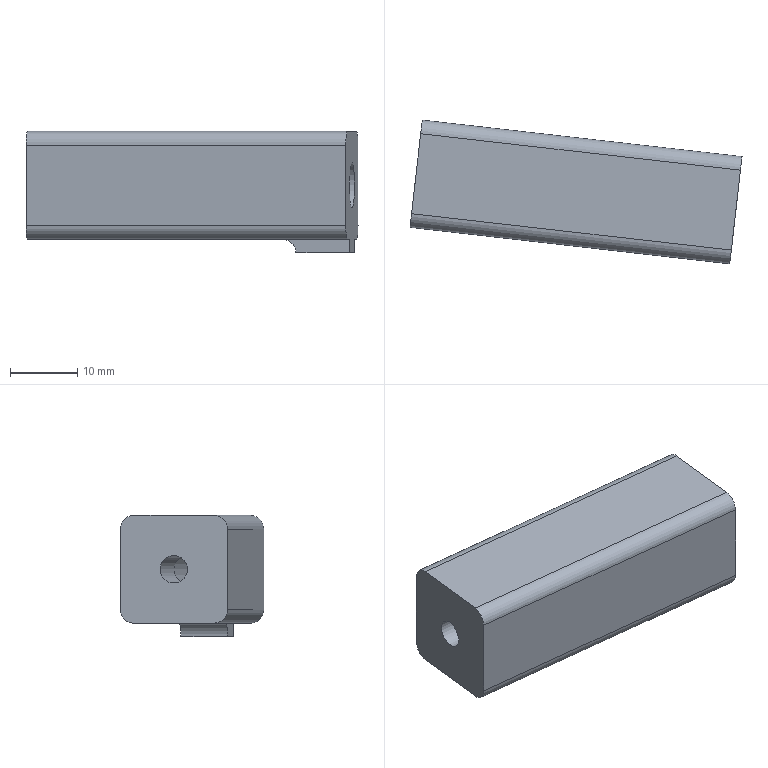Part | NX | features XQ 2 | 1 solid | 17 faces | box 49.512 x 21.41 x 18.08 mm | volume 11031 mm3 | plane 10 | cylinder 7 | commonest cylinder face diameters 4.08 x4 4 x1 4.1 x1 6.8 x1
STEP:
#1=CARTESIAN_POINT('',(3208.888,-251.717,-66.817));
#2=VERTEX_POINT('',#1);
#3=CARTESIAN_POINT('',(3208.888,-251.717,-54.817));
#4=VERTEX_POINT('',#3);
#5=CARTESIAN_POINT('',(3208.888,-251.717,-55.317));
#6=DIRECTION('',(0.,-0.000000001,1.));
#7=VECTOR('',#6,1000.);
#8=LINE('',#5,#7);
#9=EDGE_CURVE('',#2,#4,#8,.T.);
#10=ORIENTED_EDGE('',*,*,#9,.T.);
#11=CARTESIAN_POINT('',(3209.119,-249.69,-52.777));
#12=VERTEX_POINT('',#11);
#13=CARTESIAN_POINT('',(3209.119,-249.69,-54.817));
#14=DIRECTION('',(-0.9936,0.1132,0.));
#15=DIRECTION('',(0.1132,0.9936,0.));
#16=AXIS2_PLACEMENT_3D('',#13,#14,#15);
#17=CIRCLE('',#16,2.04);
#18=EDGE_CURVE('',#4,#12,#17,.T.);
#19=ORIENTED_EDGE('',*,*,#18,.T.);
#20=CARTESIAN_POINT('',(3210.477,-237.768,-52.777));
#21=VERTEX_POINT('',#20);
#22=CARTESIAN_POINT('',(3209.176,-249.194,-52.777));
#23=DIRECTION('',(0.1132,0.9936,0.000000001));
#24=VECTOR('',#23,1000.);
#25=LINE('',#22,#24);
#26=EDGE_CURVE('',#12,#21,#25,.T.);
#27=ORIENTED_EDGE('',*,*,#26,.T.);
#28=CARTESIAN_POINT('',(3210.708,-235.741,-54.817));
#29=VERTEX_POINT('',#28);
#30=CARTESIAN_POINT('',(3210.477,-237.768,-54.817));
#31=DIRECTION('',(-0.9936,0.1132,0.));
#32=DIRECTION('',(0.1132,0.9936,0.));
#33=AXIS2_PLACEMENT_3D('',#30,#31,#32);
#34=CIRCLE('',#33,2.04);
#35=EDGE_CURVE('',#21,#29,#34,.T.);
#36=ORIENTED_EDGE('',*,*,#35,.T.);
#37=CARTESIAN_POINT('',(3210.708,-235.741,-66.817));
#38=VERTEX_POINT('',#37);
#39=CARTESIAN_POINT('',(3210.708,-235.741,-55.317));
#40=DIRECTION('',(0.,0.000000001,-1.));
#41=VECTOR('',#40,1000.);
#42=LINE('',#39,#41);
#43=EDGE_CURVE('',#29,#38,#42,.T.);
#44=ORIENTED_EDGE('',*,*,#43,.T.);
#45=CARTESIAN_POINT('',(3210.477,-237.768,-68.857));
#46=VERTEX_POINT('',#45);
#47=CARTESIAN_POINT('',(3210.477,-237.768,-66.817));
#48=DIRECTION('',(-0.9936,0.1132,0.));
#49=DIRECTION('',(0.1132,0.9936,0.));
#50=AXIS2_PLACEMENT_3D('',#47,#48,#49);
#51=CIRCLE('',#50,2.04);
#52=EDGE_CURVE('',#38,#46,#51,.T.);
#53=ORIENTED_EDGE('',*,*,#52,.T.);
#54=CARTESIAN_POINT('',(3209.119,-249.69,-68.857));
#55=VERTEX_POINT('',#54);
#56=CARTESIAN_POINT('',(3209.176,-249.194,-68.857));
#57=DIRECTION('',(-0.1132,-0.9936,0.));
#58=VECTOR('',#57,1000.);
#59=LINE('',#56,#58);
#60=EDGE_CURVE('',#46,#55,#59,.T.);
#61=ORIENTED_EDGE('',*,*,#60,.T.);
#62=CARTESIAN_POINT('',(3209.119,-249.69,-66.817));
#63=DIRECTION('',(-0.9936,0.1132,0.));
#64=DIRECTION('',(0.1132,0.9936,0.));
#65=AXIS2_PLACEMENT_3D('',#62,#63,#64);
#66=CIRCLE('',#65,2.04);
#67=EDGE_CURVE('',#55,#2,#66,.T.);
#68=ORIENTED_EDGE('',*,*,#67,.T.);
#69=EDGE_LOOP('',(#10,#19,#27,#36,#44,#53,#61,#68));
#70=FACE_BOUND('',#69,.T.);
#71=CARTESIAN_POINT('',(3210.03,-241.692,-60.817));
#72=VERTEX_POINT('',#71);
#73=CARTESIAN_POINT('',(3209.798,-243.729,-60.817));
#74=DIRECTION('',(0.9936,-0.1132,0.));
#75=DIRECTION('',(0.1132,0.9936,0.));
#76=AXIS2_PLACEMENT_3D('',#73,#74,#75);
#77=CIRCLE('',#76,2.05);
#78=EDGE_CURVE('',#72,#72,#77,.T.);
#79=ORIENTED_EDGE('',*,*,#78,.T.);
#80=EDGE_LOOP('',(#79));
#81=FACE_BOUND('',#80,.T.);
#82=CARTESIAN_POINT('',(3209.176,-249.194,-55.317));
#83=DIRECTION('',(-0.9936,0.1132,0.));
#84=DIRECTION('',(-0.1132,-0.9936,0.));
#85=AXIS2_PLACEMENT_3D('',#82,#83,#84);
#86=PLANE('',#85);
#87=ADVANCED_FACE('',(#70,#81),#86,.T.);
#88=CARTESIAN_POINT('',(3257.105,-252.541,-60.817));
#89=VERTEX_POINT('',#88);
#90=CARTESIAN_POINT('',(3257.49,-249.163,-60.817));
#91=DIRECTION('',(0.9936,-0.1132,0.));
#92=DIRECTION('',(-0.1132,-0.9936,0.));
#93=AXIS2_PLACEMENT_3D('',#90,#91,#92);
#94=CIRCLE('',#93,3.4);
#95=EDGE_CURVE('',#89,#89,#94,.T.);
#96=ORIENTED_EDGE('',*,*,#95,.F.);
#97=EDGE_LOOP('',(#96));
#98=FACE_BOUND('',#97,.T.);
#99=CARTESIAN_POINT('',(3256.579,-257.151,-66.817));
#100=VERTEX_POINT('',#99);
#101=CARTESIAN_POINT('',(3256.579,-257.151,-54.817));
#102=VERTEX_POINT('',#101);
#103=CARTESIAN_POINT('',(3256.579,-257.151,-66.817));
#104=DIRECTION('',(0.,-0.000000001,1.));
#105=VECTOR('',#104,1000.);
#106=LINE('',#103,#105);
#107=EDGE_CURVE('',#100,#102,#106,.T.);
#108=ORIENTED_EDGE('',*,*,#107,.F.);
#109=CARTESIAN_POINT('',(3256.81,-255.124,-68.857));
#110=VERTEX_POINT('',#109);
#111=CARTESIAN_POINT('',(3256.81,-255.124,-66.817));
#112=DIRECTION('',(-0.9936,0.1132,0.));
#113=DIRECTION('',(-0.1132,-0.9936,0.));
#114=AXIS2_PLACEMENT_3D('',#111,#112,#113);
#115=CIRCLE('',#114,2.04);
#116=EDGE_CURVE('',#110,#100,#115,.T.);
#117=ORIENTED_EDGE('',*,*,#116,.F.);
#118=CARTESIAN_POINT('',(3257.093,-252.64,-68.857));
#119=VERTEX_POINT('',#118);
#120=CARTESIAN_POINT('',(3258.112,-243.698,-68.857));
#121=DIRECTION('',(-0.1132,-0.9936,0.));
#122=VECTOR('',#121,1000.);
#123=LINE('',#120,#122);
#124=EDGE_CURVE('',#119,#110,#123,.T.);
#125=ORIENTED_EDGE('',*,*,#124,.F.);
#126=CARTESIAN_POINT('',(3257.093,-252.64,-70.857));
#127=VERTEX_POINT('',#126);
#128=CARTESIAN_POINT('',(3257.093,-252.64,-68.892));
#129=DIRECTION('',(0.,0.,-1.));
#130=VECTOR('',#129,1000.);
#131=LINE('',#128,#130);
#132=EDGE_CURVE('',#119,#127,#131,.T.);
#133=ORIENTED_EDGE('',*,*,#132,.T.);
#134=CARTESIAN_POINT('',(3257.886,-245.685,-70.857));
#135=VERTEX_POINT('',#134);
#136=CARTESIAN_POINT('',(3258.112,-243.698,-70.857));
#137=DIRECTION('',(-0.1132,-0.9936,0.));
#138=VECTOR('',#137,1000.);
#139=LINE('',#136,#138);
#140=EDGE_CURVE('',#135,#127,#139,.T.);
#141=ORIENTED_EDGE('',*,*,#140,.F.);
#142=CARTESIAN_POINT('',(3257.886,-245.685,-68.857));
#143=VERTEX_POINT('',#142);
#144=CARTESIAN_POINT('',(3257.886,-245.685,-68.892));
#145=DIRECTION('',(0.,0.,-1.));
#146=VECTOR('',#145,1000.);
#147=LINE('',#144,#146);
#148=EDGE_CURVE('',#143,#135,#147,.T.);
#149=ORIENTED_EDGE('',*,*,#148,.F.);
#150=CARTESIAN_POINT('',(3258.169,-243.201,-68.857));
#151=VERTEX_POINT('',#150);
#152=CARTESIAN_POINT('',(3258.112,-243.698,-68.857));
#153=DIRECTION('',(-0.1132,-0.9936,0.));
#154=VECTOR('',#153,1000.);
#155=LINE('',#152,#154);
#156=EDGE_CURVE('',#151,#143,#155,.T.);
#157=ORIENTED_EDGE('',*,*,#156,.F.);
#158=CARTESIAN_POINT('',(3258.4,-241.174,-66.817));
#159=VERTEX_POINT('',#158);
#160=CARTESIAN_POINT('',(3258.169,-243.201,-66.817));
#161=DIRECTION('',(-0.9936,0.1132,0.));
#162=DIRECTION('',(-0.1132,-0.9936,0.));
#163=AXIS2_PLACEMENT_3D('',#160,#161,#162);
#164=CIRCLE('',#163,2.04);
#165=EDGE_CURVE('',#159,#151,#164,.T.);
#166=ORIENTED_EDGE('',*,*,#165,.F.);
#167=CARTESIAN_POINT('',(3258.4,-241.174,-54.817));
#168=VERTEX_POINT('',#167);
#169=CARTESIAN_POINT('',(3258.4,-241.174,-54.817));
#170=DIRECTION('',(0.,0.000000001,-1.));
#171=VECTOR('',#170,1000.);
#172=LINE('',#169,#171);
#173=EDGE_CURVE('',#168,#159,#172,.T.);
#174=ORIENTED_EDGE('',*,*,#173,.F.);
#175=CARTESIAN_POINT('',(3258.169,-243.201,-52.777));
#176=VERTEX_POINT('',#175);
#177=CARTESIAN_POINT('',(3258.169,-243.201,-54.817));
#178=DIRECTION('',(-0.9936,0.1132,0.));
#179=DIRECTION('',(-0.1132,-0.9936,0.));
#180=AXIS2_PLACEMENT_3D('',#177,#178,#179);
#181=CIRCLE('',#180,2.04);
#182=EDGE_CURVE('',#176,#168,#181,.T.);
#183=ORIENTED_EDGE('',*,*,#182,.F.);
#184=CARTESIAN_POINT('',(3256.81,-255.124,-52.777));
#185=VERTEX_POINT('',#184);
#186=CARTESIAN_POINT('',(3256.81,-255.124,-52.777));
#187=DIRECTION('',(0.1132,0.9936,0.000000001));
#188=VECTOR('',#187,1000.);
#189=LINE('',#186,#188);
#190=EDGE_CURVE('',#185,#176,#189,.T.);
#191=ORIENTED_EDGE('',*,*,#190,.F.);
#192=CARTESIAN_POINT('',(3256.81,-255.124,-54.817));
#193=DIRECTION('',(-0.9936,0.1132,0.));
#194=DIRECTION('',(-0.1132,-0.9936,0.));
#195=AXIS2_PLACEMENT_3D('',#192,#193,#194);
#196=CIRCLE('',#195,2.04);
#197=EDGE_CURVE('',#102,#185,#196,.T.);
#198=ORIENTED_EDGE('',*,*,#197,.F.);
#199=EDGE_LOOP('',(#108,#117,#125,#133,#141,#149,#157,#166,#174,#183,#191,#198));
#200=FACE_BOUND('',#199,.T.);
#201=CARTESIAN_POINT('',(3266.041,-174.108,-78.616));
#202=DIRECTION('',(0.9936,-0.1132,0.));
#203=DIRECTION('',(-0.1132,-0.9936,0.));
#204=AXIS2_PLACEMENT_3D('',#201,#202,#203);
#205=PLANE('',#204);
#206=ADVANCED_FACE('',(#98,#200),#205,.T.);
#207=CARTESIAN_POINT('',(3296.322,-261.679,-66.817));
#208=DIRECTION('',(-0.9936,0.1132,0.));
#209=VECTOR('',#208,1000.);
#210=LINE('',#207,#209);
#211=EDGE_CURVE('',#100,#2,#210,.T.);
#212=ORIENTED_EDGE('',*,*,#211,.F.);
#213=ORIENTED_EDGE('',*,*,#107,.T.);
#214=CARTESIAN_POINT('',(3205.907,-251.378,-54.817));
#215=DIRECTION('',(-0.9936,0.1132,0.000000001));
#216=VECTOR('',#215,1000.);
#217=LINE('',#214,#216);
#218=EDGE_CURVE('',#102,#4,#217,.T.);
#219=ORIENTED_EDGE('',*,*,#218,.T.);
#220=ORIENTED_EDGE('',*,*,#9,.F.);
#221=EDGE_LOOP('',(#212,#213,#219,#220));
#222=FACE_BOUND('',#221,.T.);
#223=CARTESIAN_POINT('',(3205.907,-251.378,-66.817));
#224=DIRECTION('',(-0.1132,-0.9936,-0.000000001));
#225=DIRECTION('',(0.9936,-0.1132,0.));
#226=AXIS2_PLACEMENT_3D('',#223,#224,#225);
#227=PLANE('',#226);
#228=ADVANCED_FACE('',(#222),#227,.T.);
#229=ORIENTED_EDGE('',*,*,#218,.F.);
#230=ORIENTED_EDGE('',*,*,#197,.T.);
#231=CARTESIAN_POINT('',(3206.138,-249.351,-52.777));
#232=DIRECTION('',(-0.9936,0.1132,0.000000001));
#233=VECTOR('',#232,1000.);
#234=LINE('',#231,#233);
#235=EDGE_CURVE('',#185,#12,#234,.T.);
#236=ORIENTED_EDGE('',*,*,#235,.T.);
#237=ORIENTED_EDGE('',*,*,#18,.F.);
#238=EDGE_LOOP('',(#229,#230,#236,#237));
#239=FACE_BOUND('',#238,.T.);
#240=CARTESIAN_POINT('',(3206.138,-249.351,-54.817));
#241=DIRECTION('',(-0.9936,0.1132,0.000000001));
#242=DIRECTION('',(-0.1132,-0.9936,0.));
#243=AXIS2_PLACEMENT_3D('',#240,#241,#242);
#244=CYLINDRICAL_SURFACE('',#243,2.04);
#245=ADVANCED_FACE('',(#239),#244,.T.);
#246=ORIENTED_EDGE('',*,*,#235,.F.);
#247=ORIENTED_EDGE('',*,*,#190,.T.);
#248=CARTESIAN_POINT('',(3207.497,-237.428,-52.777));
#249=DIRECTION('',(-0.9936,0.1132,0.000000001));
#250=VECTOR('',#249,1000.);
#251=LINE('',#248,#250);
#252=EDGE_CURVE('',#176,#21,#251,.T.);
#253=ORIENTED_EDGE('',*,*,#252,.T.);
#254=ORIENTED_EDGE('',*,*,#26,.F.);
#255=EDGE_LOOP('',(#246,#247,#253,#254));
#256=FACE_BOUND('',#255,.T.);
#257=CARTESIAN_POINT('',(3206.138,-249.351,-52.777));
#258=DIRECTION('',(0.000000001,-0.000000002,1.));
#259=DIRECTION('',(0.225,0.9744,0.000000001));
#260=AXIS2_PLACEMENT_3D('',#257,#258,#259);
#261=PLANE('',#260);
#262=ADVANCED_FACE('',(#256),#261,.T.);
#263=ORIENTED_EDGE('',*,*,#252,.F.);
#264=ORIENTED_EDGE('',*,*,#182,.T.);
#265=CARTESIAN_POINT('',(3207.728,-235.401,-54.817));
#266=DIRECTION('',(-0.9936,0.1132,0.000000001));
#267=VECTOR('',#266,1000.);
#268=LINE('',#265,#267);
#269=EDGE_CURVE('',#168,#29,#268,.T.);
#270=ORIENTED_EDGE('',*,*,#269,.T.);
#271=ORIENTED_EDGE('',*,*,#35,.F.);
#272=EDGE_LOOP('',(#263,#264,#270,#271));
#273=FACE_BOUND('',#272,.T.);
#274=CARTESIAN_POINT('',(3207.497,-237.428,-54.817));
#275=DIRECTION('',(-0.9936,0.1132,0.000000001));
#276=DIRECTION('',(-0.1132,-0.9936,0.));
#277=AXIS2_PLACEMENT_3D('',#274,#275,#276);
#278=CYLINDRICAL_SURFACE('',#277,2.04);
#279=ADVANCED_FACE('',(#273),#278,.T.);
#280=ORIENTED_EDGE('',*,*,#269,.F.);
#281=ORIENTED_EDGE('',*,*,#173,.T.);
#282=CARTESIAN_POINT('',(3233.064,-238.288,-66.817));
#283=DIRECTION('',(-0.9936,0.1132,0.000000001));
#284=VECTOR('',#283,1000.);
#285=LINE('',#282,#284);
#286=EDGE_CURVE('',#159,#38,#285,.T.);
#287=ORIENTED_EDGE('',*,*,#286,.T.);
#288=ORIENTED_EDGE('',*,*,#43,.F.);
#289=EDGE_LOOP('',(#280,#281,#287,#288));
#290=FACE_BOUND('',#289,.T.);
#291=CARTESIAN_POINT('',(3207.728,-235.401,-54.817));
#292=DIRECTION('',(0.1132,0.9936,0.000000001));
#293=DIRECTION('',(-0.9936,0.1132,0.));
#294=AXIS2_PLACEMENT_3D('',#291,#292,#293);
#295=PLANE('',#294);
#296=ADVANCED_FACE('',(#290),#295,.T.);
#297=ORIENTED_EDGE('',*,*,#286,.F.);
#298=ORIENTED_EDGE('',*,*,#165,.T.);
#299=CARTESIAN_POINT('',(3207.497,-237.428,-68.857));
#300=DIRECTION('',(-0.9936,0.1132,0.000000001));
#301=VECTOR('',#300,1000.);
#302=LINE('',#299,#301);
#303=EDGE_CURVE('',#151,#46,#302,.T.);
#304=ORIENTED_EDGE('',*,*,#303,.T.);
#305=ORIENTED_EDGE('',*,*,#52,.F.);
#306=EDGE_LOOP('',(#297,#298,#304,#305));
#307=FACE_BOUND('',#306,.T.);
#308=CARTESIAN_POINT('',(3207.497,-237.428,-66.817));
#309=DIRECTION('',(0.9936,-0.1132,-0.000000001));
#310=DIRECTION('',(0.1132,0.9936,0.));
#311=AXIS2_PLACEMENT_3D('',#308,#309,#310);
#312=CYLINDRICAL_SURFACE('',#311,2.04);
#313=ADVANCED_FACE('',(#307),#312,.T.);
#314=CARTESIAN_POINT('',(3247.95,-244.553,-68.857));
#315=VERTEX_POINT('',#314);
#316=CARTESIAN_POINT('',(3297.629,-250.213,-68.857));
#317=DIRECTION('',(-0.9936,0.1132,0.));
#318=VECTOR('',#317,1000.);
#319=LINE('',#316,#318);
#320=EDGE_CURVE('',#143,#315,#319,.T.);
#321=ORIENTED_EDGE('',*,*,#320,.T.);
#322=CARTESIAN_POINT('',(3247.158,-251.508,-68.857));
#323=VERTEX_POINT('',#322);
#324=CARTESIAN_POINT('',(3247.158,-251.508,-68.857));
#325=DIRECTION('',(-0.1132,-0.9936,0.));
#326=VECTOR('',#325,1000.);
#327=LINE('',#324,#326);
#328=EDGE_CURVE('',#315,#323,#327,.T.);
#329=ORIENTED_EDGE('',*,*,#328,.T.);
#330=CARTESIAN_POINT('',(3296.836,-257.168,-68.857));
#331=DIRECTION('',(-0.9936,0.1132,0.));
#332=VECTOR('',#331,1000.);
#333=LINE('',#330,#332);
#334=EDGE_CURVE('',#119,#323,#333,.T.);
#335=ORIENTED_EDGE('',*,*,#334,.F.);
#336=ORIENTED_EDGE('',*,*,#124,.T.);
#337=CARTESIAN_POINT('',(3296.553,-259.652,-68.857));
#338=DIRECTION('',(-0.9936,0.1132,0.));
#339=VECTOR('',#338,1000.);
#340=LINE('',#337,#339);
#341=EDGE_CURVE('',#110,#55,#340,.T.);
#342=ORIENTED_EDGE('',*,*,#341,.T.);
#343=ORIENTED_EDGE('',*,*,#60,.F.);
#344=ORIENTED_EDGE('',*,*,#303,.F.);
#345=ORIENTED_EDGE('',*,*,#156,.T.);
#346=EDGE_LOOP('',(#321,#329,#335,#336,#342,#343,#344,#345));
#347=FACE_BOUND('',#346,.T.);
#348=CARTESIAN_POINT('',(3297.855,-248.226,-68.857));
#349=DIRECTION('',(0.,0.,-1.));
#350=DIRECTION('',(0.06105,-0.9981,0.));
#351=AXIS2_PLACEMENT_3D('',#348,#349,#350);
#352=PLANE('',#351);
#353=ADVANCED_FACE('',(#347),#352,.T.);
#354=ORIENTED_EDGE('',*,*,#341,.F.);
#355=ORIENTED_EDGE('',*,*,#116,.T.);
#356=ORIENTED_EDGE('',*,*,#211,.T.);
#357=ORIENTED_EDGE('',*,*,#67,.F.);
#358=EDGE_LOOP('',(#354,#355,#356,#357));
#359=FACE_BOUND('',#358,.T.);
#360=CARTESIAN_POINT('',(3296.553,-259.652,-66.817));
#361=DIRECTION('',(-0.9936,0.1132,0.));
#362=DIRECTION('',(-0.1132,-0.9936,0.));
#363=AXIS2_PLACEMENT_3D('',#360,#361,#362);
#364=CYLINDRICAL_SURFACE('',#363,2.04);
#365=ADVANCED_FACE('',(#359),#364,.T.);
#366=ORIENTED_EDGE('',*,*,#334,.T.);
#367=CARTESIAN_POINT('',(3249.145,-251.735,-70.857));
#368=VERTEX_POINT('',#367);
#369=CARTESIAN_POINT('',(3247.158,-251.508,-70.857));
#370=DIRECTION('',(0.1132,0.9936,0.));
#371=DIRECTION('',(-0.9936,0.1132,0.));
#372=AXIS2_PLACEMENT_3D('',#369,#370,#371);
#373=CIRCLE('',#372,2.);
#374=EDGE_CURVE('',#323,#368,#373,.T.);
#375=ORIENTED_EDGE('',*,*,#374,.T.);
#376=CARTESIAN_POINT('',(3296.836,-257.168,-70.857));
#377=DIRECTION('',(-0.9936,0.1132,0.));
#378=VECTOR('',#377,1000.);
#379=LINE('',#376,#378);
#380=EDGE_CURVE('',#127,#368,#379,.T.);
#381=ORIENTED_EDGE('',*,*,#380,.F.);
#382=ORIENTED_EDGE('',*,*,#132,.F.);
#383=EDGE_LOOP('',(#366,#375,#381,#382));
#384=FACE_BOUND('',#383,.T.);
#385=CARTESIAN_POINT('',(3296.836,-257.168,-68.892));
#386=DIRECTION('',(-0.1132,-0.9936,0.));
#387=DIRECTION('',(-0.9936,0.1132,0.));
#388=AXIS2_PLACEMENT_3D('',#385,#386,#387);
#389=PLANE('',#388);
#390=ADVANCED_FACE('',(#384),#389,.T.);
#391=CARTESIAN_POINT('',(3249.937,-244.78,-70.857));
#392=VERTEX_POINT('',#391);
#393=CARTESIAN_POINT('',(3297.629,-250.213,-70.857));
#394=DIRECTION('',(-0.9936,0.1132,0.));
#395=VECTOR('',#394,1000.);
#396=LINE('',#393,#395);
#397=EDGE_CURVE('',#135,#392,#396,.T.);
#398=ORIENTED_EDGE('',*,*,#397,.T.);
#399=CARTESIAN_POINT('',(3247.95,-244.553,-70.857));
#400=DIRECTION('',(-0.1132,-0.9936,0.));
#401=DIRECTION('',(-0.9936,0.1132,0.));
#402=AXIS2_PLACEMENT_3D('',#399,#400,#401);
#403=CIRCLE('',#402,2.);
#404=EDGE_CURVE('',#392,#315,#403,.T.);
#405=ORIENTED_EDGE('',*,*,#404,.T.);
#406=ORIENTED_EDGE('',*,*,#320,.F.);
#407=ORIENTED_EDGE('',*,*,#148,.T.);
#408=EDGE_LOOP('',(#398,#405,#406,#407));
#409=FACE_BOUND('',#408,.T.);
#410=CARTESIAN_POINT('',(3297.629,-250.213,-68.892));
#411=DIRECTION('',(-0.1132,-0.9936,0.));
#412=DIRECTION('',(-0.9936,0.1132,0.));
#413=AXIS2_PLACEMENT_3D('',#410,#411,#412);
#414=PLANE('',#413);
#415=ADVANCED_FACE('',(#409),#414,.F.);
#416=ORIENTED_EDGE('',*,*,#380,.T.);
#417=CARTESIAN_POINT('',(3250.164,-242.792,-70.857));
#418=DIRECTION('',(0.1132,0.9936,0.));
#419=VECTOR('',#418,1000.);
#420=LINE('',#417,#419);
#421=EDGE_CURVE('',#368,#392,#420,.T.);
#422=ORIENTED_EDGE('',*,*,#421,.T.);
#423=ORIENTED_EDGE('',*,*,#397,.F.);
#424=ORIENTED_EDGE('',*,*,#140,.T.);
#425=EDGE_LOOP('',(#416,#422,#423,#424));
#426=FACE_BOUND('',#425,.T.);
#427=CARTESIAN_POINT('',(3297.855,-248.226,-70.857));
#428=DIRECTION('',(0.,0.,-1.));
#429=DIRECTION('',(0.06105,-0.9981,0.));
#430=AXIS2_PLACEMENT_3D('',#427,#428,#429);
#431=PLANE('',#430);
#432=ADVANCED_FACE('',(#426),#431,.T.);
#433=ORIENTED_EDGE('',*,*,#374,.F.);
#434=ORIENTED_EDGE('',*,*,#328,.F.);
#435=ORIENTED_EDGE('',*,*,#404,.F.);
#436=ORIENTED_EDGE('',*,*,#421,.F.);
#437=EDGE_LOOP('',(#433,#434,#435,#436));
#438=FACE_BOUND('',#437,.T.);
#439=CARTESIAN_POINT('',(3247.554,-248.031,-70.857));
#440=DIRECTION('',(-0.1132,-0.9936,0.));
#441=DIRECTION('',(-0.9936,0.1132,0.));
#442=AXIS2_PLACEMENT_3D('',#439,#440,#441);
#443=CYLINDRICAL_SURFACE('',#442,2.);
#444=ADVANCED_FACE('',(#438),#443,.F.);
#445=ORIENTED_EDGE('',*,*,#95,.T.);
#446=EDGE_LOOP('',(#445));
#447=FACE_BOUND('',#446,.T.);
#448=CARTESIAN_POINT('',(3228.067,-242.389,-60.817));
#449=VERTEX_POINT('',#448);
#450=CARTESIAN_POINT('',(3227.682,-245.767,-60.817));
#451=DIRECTION('',(0.9936,-0.1132,0.));
#452=DIRECTION('',(0.1132,0.9936,0.));
#453=AXIS2_PLACEMENT_3D('',#450,#451,#452);
#454=CIRCLE('',#453,3.4);
#455=EDGE_CURVE('',#449,#449,#454,.T.);
#456=ORIENTED_EDGE('',*,*,#455,.F.);
#457=EDGE_LOOP('',(#456));
#458=FACE_BOUND('',#457,.T.);
#459=CARTESIAN_POINT('',(3267.425,-250.295,-60.817));
#460=DIRECTION('',(-0.9936,0.1132,0.));
#461=DIRECTION('',(0.1132,0.9936,0.));
#462=AXIS2_PLACEMENT_3D('',#459,#460,#461);
#463=CYLINDRICAL_SURFACE('',#462,3.4);
#464=ADVANCED_FACE('',(#447,#458),#463,.F.);
#465=CARTESIAN_POINT('',(3227.915,-243.73,-60.817));
#466=VERTEX_POINT('',#465);
#467=CARTESIAN_POINT('',(3227.682,-245.767,-60.817));
#468=DIRECTION('',(0.9936,-0.1132,0.));
#469=DIRECTION('',(0.1132,0.9936,0.));
#470=AXIS2_PLACEMENT_3D('',#467,#468,#469);
#471=CIRCLE('',#470,2.05);
#472=EDGE_CURVE('',#466,#466,#471,.T.);
#473=ORIENTED_EDGE('',*,*,#472,.F.);
#474=EDGE_LOOP('',(#473));
#475=FACE_BOUND('',#474,.T.);
#476=ORIENTED_EDGE('',*,*,#455,.T.);
#477=EDGE_LOOP('',(#476));
#478=FACE_BOUND('',#477,.T.);
#479=CARTESIAN_POINT('',(3227.682,-245.767,-60.817));
#480=DIRECTION('',(-0.9936,0.1132,0.));
#481=DIRECTION('',(0.1132,0.9936,0.));
#482=AXIS2_PLACEMENT_3D('',#479,#480,#481);
#483=PLANE('',#482);
#484=ADVANCED_FACE('',(#475,#478),#483,.F.);
#485=ORIENTED_EDGE('',*,*,#78,.F.);
#486=EDGE_LOOP('',(#485));
#487=FACE_BOUND('',#486,.T.);
#488=ORIENTED_EDGE('',*,*,#472,.T.);
#489=EDGE_LOOP('',(#488));
#490=FACE_BOUND('',#489,.T.);
#491=CARTESIAN_POINT('',(3205.824,-243.276,-60.817));
#492=DIRECTION('',(0.9936,-0.1132,0.));
#493=DIRECTION('',(-0.1132,-0.9936,0.));
#494=AXIS2_PLACEMENT_3D('',#491,#492,#493);
#495=CYLINDRICAL_SURFACE('',#494,2.05);
#496=ADVANCED_FACE('',(#487,#490),#495,.F.);
#497=CLOSED_SHELL('',(#87,#206,#228,#245,#262,#279,#296,#313,#353,#365,#390,#415,#432,#444,#464,#484,#496));
#498=MANIFOLD_SOLID_BREP('',#497);
#499=(LENGTH_UNIT()NAMED_UNIT(*)SI_UNIT(.MILLI.,.METRE.));
#500=UNCERTAINTY_MEASURE_WITH_UNIT(LENGTH_MEASURE(0.00001),#499,'','');
#501=(NAMED_UNIT(*)PLANE_ANGLE_UNIT()SI_UNIT($,.RADIAN.));
#502=(NAMED_UNIT(*)SI_UNIT($,.STERADIAN.)SOLID_ANGLE_UNIT());
#503=(GEOMETRIC_REPRESENTATION_CONTEXT(3)GLOBAL_UNCERTAINTY_ASSIGNED_CONTEXT((#500))GLOBAL_UNIT_ASSIGNED_CONTEXT((#499,#501,#502))REPRESENTATION_CONTEXT('',''));
#504=ADVANCED_BREP_SHAPE_REPRESENTATION('',(#498),#503);